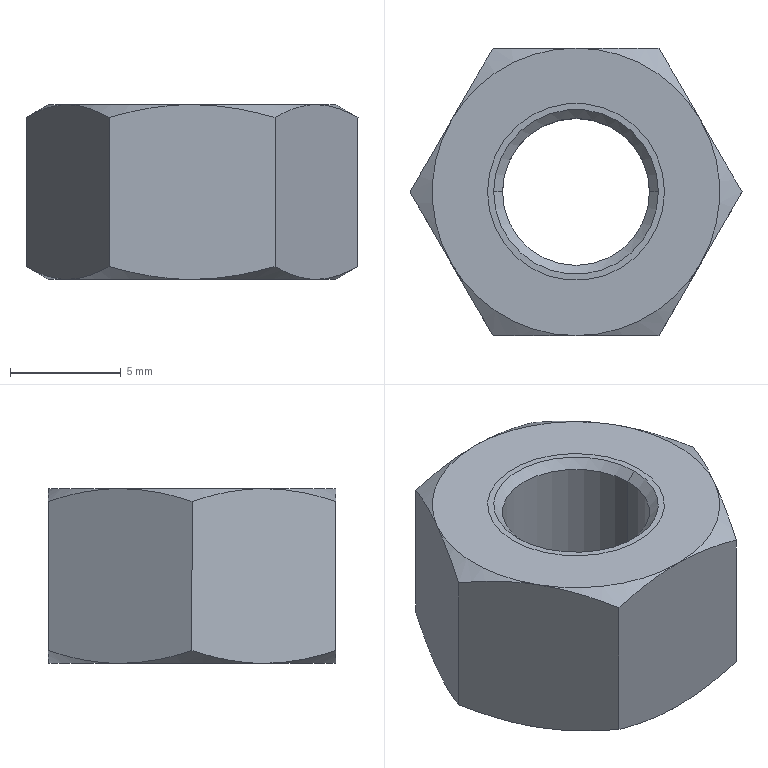Part | NX | features BREP 2 | 1 solid | 28 faces | box 15.011 x 13 x 7.9 mm | volume 1139 mm3 | cone 16 | plane 8 | cylinder 4 | commonest cylinder face diameters 6.647 x2 8 x2